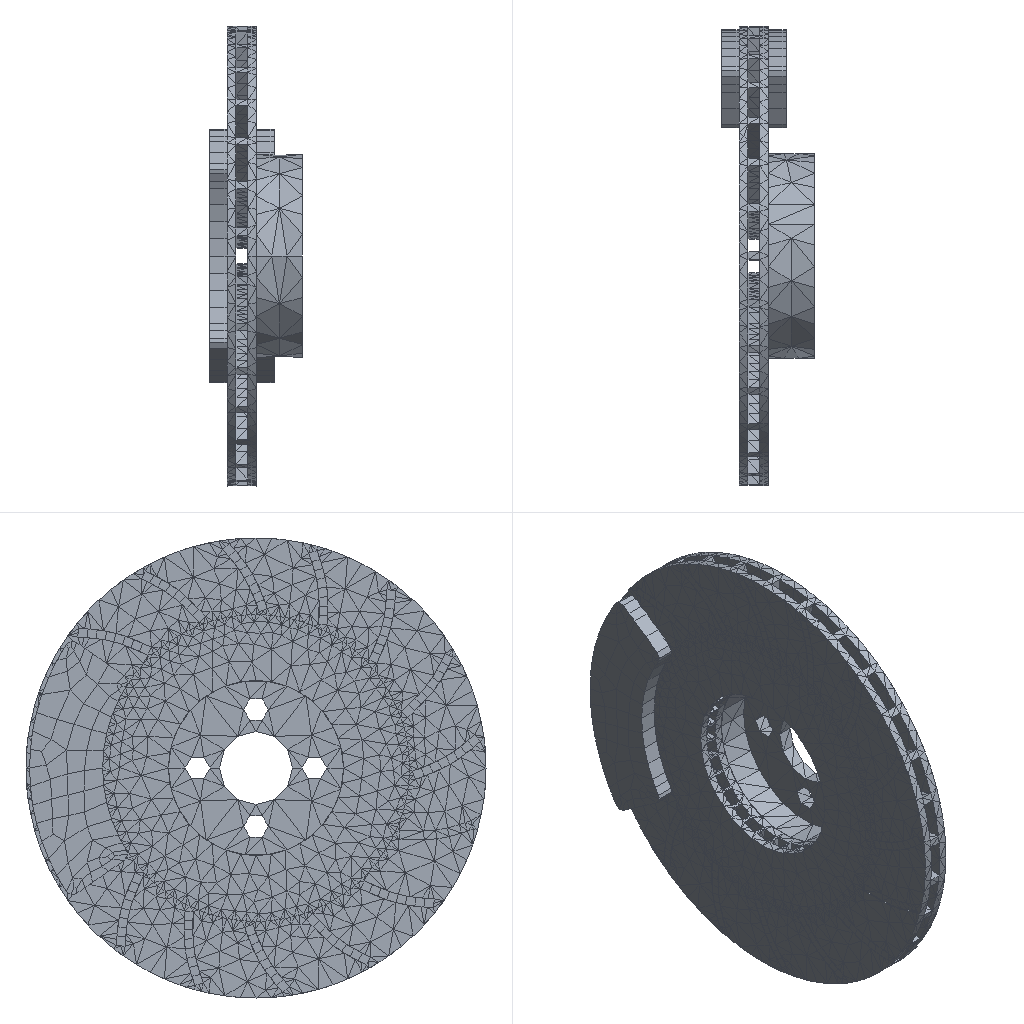Simulation study | ansys workbench
Ansys APDL input file, long lists of numbers shortened:
/batch
/config,noeldb,1     ! force off writing results to database
*get,_wallstrt,active,,time,wall
! ANSYS input file written by Workbench version 2022 R1
! File used for geometry attach:
/title,1111--___ (B5)
! ****** Begin Custom Load Command Snippet ******
/COM, ACT Extensions:
/COM,     LSDYNA, 2021.1
/COM,
! ****** End   Custom Load Command Snippet ******
*DIM,_wb_ProjectScratch_dir,string,248
_wb_ProjectScratch_dir(1) = ''
*DIM,_wb_SolverFiles_dir,string,248
_wb_SolverFiles_dir(1) = ''
*DIM,_wb_userfiles_dir,string,248
_wb_userfiles_dir(1) = ''
/com,--- Data in consistent NMM units. See Solving Units in the help system for more information.
/units,MPA
/nopr
/wb,file,start              !  signify a WB generated input file
/prep7
! Turn off shape checking because checks already performed inside WB mesher.
! See help system for more information.
SHPP,OFF,,NOWARN
/nolist
etcon,set             ! allow ANSYS to choose best KEYOP's for 180x elements, resets any applicable keyopt to MAPDL defaults
/com,*********** Nodes for the whole assembly ***********
nblock,3,,31611
(1i9,3e20.9e3)
        1    -5.687067418E+00     4.219548714E+00     4.362788327E+02
! (28737 more lines like these left out)
-1
/wb,elem,start            !  set before creation of elements
/com,*********** Elements for Body 1 "model|____-____/____1" ***********
et,1,279
eblock,19,solid,,71
(19i9)
        1        1        1        1        0        0        0        0       20        0      113     1461     1475     1498     1507     1554     1540     1517     1508
! (141 more lines like these left out)
-1
/com,*********** Elements for Body 2 "model|____-____/____1[2]" ***********
et,2,279
eblock,19,solid,,75
(19i9)
        2        2        2        2        0        0        0        0       20        0      184     2069     2116     2084     2070     2164     2117     2149     2163
! (149 more lines like these left out)
-1
/com,*********** Elements for Body 3 "model|____-____3[1]" ***********
et,3,291
eblock,19,solid,,12722
(19i9)
        3        3        3        3        0        0        0        0       10        0      763     6344     7992     7917     7984    24419    28694    24417    24418
! (25443 more lines like these left out)
-1
/com,*********** Elements for Body 4 "model|____-____3[2]" ***********
et,4,291
eblock,19,solid,,496
(19i9)
        4        4        4        4        0        0        0        0       10        0      267     2871     3008     2982     3017     3464     3916     3463     3465
! (991 more lines like these left out)
-1
/com,*********** Elements for Body 5 "model|Solid" ***********
et,5,279
eblock,19,solid,,8
(19i9)
        5        5        5        5        0        0        0        0       20        0       33      417      426      425      424      452      437      444      445
! (15 more lines like these left out)
-1
! (14 more sections like these left out)
/wb,elem,end               !  done creating elements
/com,*********** Send User Defined Coordinate System(s) ***********
csys,0
toffst,273.15,  ! Temperature offset from absolute zero
/wb,mat,start              !  starting to send materials
/com,*********** Send Materials ***********
Temperature = 'TEMP' ! Temperature
MP,DENS,1,7.85e-09,	! tonne mm^-3
MP,ALPX,1,1.2e-05,	! C^-1
MP,C,1,434000000,	! mm^2 s^-2 C^-1
MP,KXX,1,60.5,	! tonne mm s^-3 C^-1
MP,RSVX,1,0.00017,	! ohm mm
MP,EX,1,200000,	! tonne s^-2 mm^-1
MP,NUXY,1,0.3,
MP,MURX,1,10000,
Temperature = 'TEMP' ! Temperature
MP,DENS,2,7.85e-09,	! tonne mm^-3
MP,ALPX,2,1.2e-05,	! C^-1
MP,C,2,434000000,	! mm^2 s^-2 C^-1
MP,KXX,2,60.5,	! tonne mm s^-3 C^-1
MP,RSVX,2,0.00017,	! ohm mm
MP,EX,2,200000,	! tonne s^-2 mm^-1
MP,NUXY,2,0.3,
MP,MURX,2,10000,
Temperature = 'TEMP' ! Temperature
MP,DENS,3,7.85e-09,	! tonne mm^-3
MP,ALPX,3,1.2e-05,	! C^-1
MP,C,3,434000000,	! mm^2 s^-2 C^-1
MP,KXX,3,60.5,	! tonne mm s^-3 C^-1
MP,RSVX,3,0.00017,	! ohm mm
MP,EX,3,200000,	! tonne s^-2 mm^-1
MP,NUXY,3,0.3,
MP,MURX,3,10000,
Temperature = 'TEMP' ! Temperature
MP,DENS,4,7.85e-09,	! tonne mm^-3
MP,ALPX,4,1.2e-05,	! C^-1
MP,C,4,434000000,	! mm^2 s^-2 C^-1
MP,KXX,4,60.5,	! tonne mm s^-3 C^-1
MP,RSVX,4,0.00017,	! ohm mm
MP,EX,4,200000,	! tonne s^-2 mm^-1
MP,NUXY,4,0.3,
MP,MURX,4,10000,
Temperature = 'TEMP' ! Temperature
MP,DENS,5,7.85e-09,	! tonne mm^-3
MP,ALPX,5,1.2e-05,	! C^-1
MP,C,5,434000000,	! mm^2 s^-2 C^-1
MP,KXX,5,60.5,	! tonne mm s^-3 C^-1
MP,RSVX,5,0.00017,	! ohm mm
MP,EX,5,200000,	! tonne s^-2 mm^-1
MP,NUXY,5,0.3,
MP,MURX,5,10000,
Temperature = 'TEMP' ! Temperature
MP,DENS,6,7.85e-09,	! tonne mm^-3
MP,ALPX,6,1.2e-05,	! C^-1
MP,C,6,434000000,	! mm^2 s^-2 C^-1
MP,KXX,6,60.5,	! tonne mm s^-3 C^-1
MP,RSVX,6,0.00017,	! ohm mm
MP,EX,6,200000,	! tonne s^-2 mm^-1
MP,NUXY,6,0.3,
MP,MURX,6,10000,
Temperature = 'TEMP' ! Temperature
MP,DENS,7,7.85e-09,	! tonne mm^-3
MP,ALPX,7,1.2e-05,	! C^-1
MP,C,7,434000000,	! mm^2 s^-2 C^-1
MP,KXX,7,60.5,	! tonne mm s^-3 C^-1
MP,RSVX,7,0.00017,	! ohm mm
MP,EX,7,200000,	! tonne s^-2 mm^-1
MP,NUXY,7,0.3,
MP,MURX,7,10000,
Temperature = 'TEMP' ! Temperature
MP,DENS,8,7.85e-09,	! tonne mm^-3
MP,ALPX,8,1.2e-05,	! C^-1
MP,C,8,434000000,	! mm^2 s^-2 C^-1
MP,KXX,8,60.5,	! tonne mm s^-3 C^-1
MP,RSVX,8,0.00017,	! ohm mm
MP,EX,8,200000,	! tonne s^-2 mm^-1
MP,NUXY,8,0.3,
MP,MURX,8,10000,
Temperature = 'TEMP' ! Temperature
MP,DENS,9,7.85e-09,	! tonne mm^-3
MP,ALPX,9,1.2e-05,	! C^-1
MP,C,9,434000000,	! mm^2 s^-2 C^-1
MP,KXX,9,60.5,	! tonne mm s^-3 C^-1
MP,RSVX,9,0.00017,	! ohm mm
MP,EX,9,200000,	! tonne s^-2 mm^-1
! (92 more lines like these left out)
/wb,mat,end                !  done sending materials
!************************* Model Summary ********************
!model|____-____/____1,	结构钢,	matid,	1
!model|____-____/____1[2],	结构钢,	matid,	2
!model|____-____3[1],	结构钢,	matid,	3
!model|____-____3[2],	结构钢,	matid,	4
!model|Solid,	结构钢,	matid,	5
!model|Solid[2],	结构钢,	matid,	6
!model|Solid[3],	结构钢,	matid,	7
!model|Solid[4],	结构钢,	matid,	8
!model|Solid[5],	结构钢,	matid,	9
!model|Solid[6],	结构钢,	matid,	10
!model|Solid[7],	结构钢,	matid,	11
!model|Solid[8],	结构钢,	matid,	12
!model|Solid[9],	结构钢,	matid,	13
!model|Solid[10],	结构钢,	matid,	14
!model|Solid[11],	结构钢,	matid,	15
!model|Solid[12],	结构钢,	matid,	16
!model|Solid[13],	结构钢,	matid,	17
!model|Solid[14],	结构钢,	matid,	18
!model|Solid[15],	结构钢,	matid,	19
!************************* End Model Summary ********************
! get the diagonal of the bounding box. Needed later for other things
*get,_xmin,node,,mnloc,x
*get,_ymin,node,,mnloc,y
*get,_zmin,node,,mnloc,z
*get,_xmax,node,,mxloc,x
*get,_ymax,node,,mxloc,y
*get,_zmax,node,,mxloc,z
_ASMDIAG=(_xmax-_xmin)*(_xmax-_xmin)+(_ymax-_ymin)*(_ymax-_ymin)+(_zmax-_zmin)*(_zmax-_zmin)
_ASMDIAG=SQRT(_ASMDIAG)
/wb,contact,start          !  starting to send contact
/com,*********** Create Contact "接触区域" ***********
/com,            Real Constant Set For Above Contact Is 21 & 20
*set,tid,21
*set,cid,20
r,tid
r,cid
et,tid,170
et,cid,174
eblock,10,,,71
(15i9)
    22751       21       21       21        0     1554     1540     1517     1508     1908     1847     1815     1817
! (70 more lines like these left out)
-1
eblock,10,,,71
(15i9)
    22822       20       20       20        0     1554     1540     1517     1508     1908     1847     1815     1817
! (70 more lines like these left out)
-1
eblock,10,,,315
(15i9)
    22893       20       21       20        0     4246     7172     4247     4247     9933     9941     4247     9930
! (314 more lines like these left out)
-1
eblock,10,,,315
(15i9)
    23208       21       20       21        0     4246     7172     4247     4247     9933     9941     4247     9930
! (314 more lines like these left out)
-1
keyo,cid,8,2               ! auto create asymmetric contact (from Program Controlled setting)
keyo,cid,10,0              ! adjust contact stiffness each NR iteration (from Program Controlled setting)
keyo,cid,12,5              ! bonded always
keyo,cid,18,1              ! small sliding turned on by application
keyo,cid,2,0               ! augmented Lagrange (from Program Controlled setting)
keyo,cid,4,0               ! on Gauss point (from Program Controlled setting)
keyo,cid,9,1               ! ignore initial gaps/penetration
keyo,cid,7,0               ! No Prediction
rmod,tid,3,10.      ! FKN
rmod,tid,5,0.       ! ICONT
rmod,tid,6,0.       ! PINB
rmod,tid,10,0.      ! CNOF
rmod,tid,12,0.      ! FKT
rmod,tid,36,80      ! WB DSID
rmod,cid,3,10.      ! FKN
rmod,cid,5,0.       ! ICONT
rmod,cid,6,0.       ! PINB
rmod,cid,10,0.      ! CNOF
rmod,cid,12,0.      ! FKT
rmod,cid,36,80      ! WB DSID
*set,_maxkxx,605000.
rmod,cid,14,_maxkxx/_ASMDIAG         ! TCC, Divide by Length since Traction Based
rmod,tid,14,_maxkxx/_ASMDIAG      ! TCC, Divide by Length since Traction Based
keyo,cid,1,2     ! Pure thermal contact
/com,*********** Create Contact "接触区域 2" ***********
/com,            Real Constant Set For Above Contact Is 23 & 22
*set,tid,23
*set,cid,22
r,tid
r,cid
et,tid,170
et,cid,174
eblock,10,,,10
(15i9)
    23523       23       23       23        0     1512     1544     1542     1539     1831     1910     1904     1830
! (9 more lines like these left out)
-1
eblock,10,,,10
(15i9)
    23533       22       22       22        0     1512     1544     1542     1539     1831     1910     1904     1830
! (9 more lines like these left out)
-1
eblock,10,,,8
(15i9)
    23543       22       23       22        0      649      653      652      651      718      721      720      717
! (7 more lines like these left out)
-1
eblock,10,,,8
(15i9)
    23551       23       22       23        0      649      653      652      651      718      721      720      717
! (7 more lines like these left out)
-1
keyo,cid,8,2               ! auto create asymmetric contact (from Program Controlled setting)
keyo,cid,10,0              ! adjust contact stiffness each NR iteration (from Program Controlled setting)
keyo,cid,12,5              ! bonded always
keyo,cid,18,1              ! small sliding turned on by application
keyo,cid,2,0               ! augmented Lagrange (from Program Controlled setting)
keyo,cid,4,0               ! on Gauss point (from Program Controlled setting)
keyo,cid,9,1               ! ignore initial gaps/penetration
keyo,cid,7,0               ! No Prediction
rmod,tid,3,10.      ! FKN
rmod,tid,5,0.       ! ICONT
rmod,tid,6,0.       ! PINB
rmod,tid,10,0.      ! CNOF
rmod,tid,12,0.      ! FKT
rmod,tid,36,83      ! WB DSID
rmod,cid,3,10.      ! FKN
rmod,cid,5,0.       ! ICONT
rmod,cid,6,0.       ! PINB
rmod,cid,10,0.      ! CNOF
rmod,cid,12,0.      ! FKT
rmod,cid,36,83      ! WB DSID
*set,_maxkxx,605000.
rmod,cid,14,_maxkxx/_ASMDIAG         ! TCC, Divide by Length since Traction Based
rmod,tid,14,_maxkxx/_ASMDIAG      ! TCC, Divide by Length since Traction Based
keyo,cid,1,2     ! Pure thermal contact
/com,*********** Create Contact "接触区域 3" ***********
/com,            Real Constant Set For Above Contact Is 25 & 24
*set,tid,25
*set,cid,24
r,tid
r,cid
et,tid,170
et,cid,174
eblock,10,,,11
(15i9)
    23559       25       25       25        0     1529     1530     1531     1532     1881     1884     1887     1882
! (10 more lines like these left out)
-1
eblock,10,,,11
(15i9)
    23570       24       24       24        0     1529     1530     1531     1532     1881     1884     1887     1882
! (10 more lines like these left out)
-1
eblock,10,,,8
(15i9)
    23581       24       25       24        0      972      957      964      965     1021     1020     1033     1034
! (7 more lines like these left out)
-1
eblock,10,,,8
(15i9)
    23589       25       24       25        0      972      957      964      965     1021     1020     1033     1034
! (7 more lines like these left out)
-1
keyo,cid,8,2               ! auto create asymmetric contact (from Program Controlled setting)
keyo,cid,10,0              ! adjust contact stiffness each NR iteration (from Program Controlled setting)
keyo,cid,12,5              ! bonded always
keyo,cid,18,1              ! small sliding turned on by application
keyo,cid,2,0               ! augmented Lagrange (from Program Controlled setting)
keyo,cid,4,0               ! on Gauss point (from Program Controlled setting)
keyo,cid,9,1               ! ignore initial gaps/penetration
keyo,cid,7,0               ! No Prediction
rmod,tid,3,10.      ! FKN
rmod,tid,5,0.       ! ICONT
rmod,tid,6,0.       ! PINB
rmod,tid,10,0.      ! CNOF
rmod,tid,12,0.      ! FKT
rmod,tid,36,86      ! WB DSID
rmod,cid,3,10.      ! FKN
rmod,cid,5,0.       ! ICONT
rmod,cid,6,0.       ! PINB
rmod,cid,10,0.      ! CNOF
rmod,cid,12,0.      ! FKT
rmod,cid,36,86      ! WB DSID
*set,_maxkxx,605000.
rmod,cid,14,_maxkxx/_ASMDIAG         ! TCC, Divide by Length since Traction Based
rmod,tid,14,_maxkxx/_ASMDIAG      ! TCC, Divide by Length since Traction Based
keyo,cid,1,2     ! Pure thermal contact
/com,*********** Create Contact "接触区域 4" ***********
/com,            Real Constant Set For Above Contact Is 27 & 26
*set,tid,27
*set,cid,26
r,tid
r,cid
et,tid,170
et,cid,174
eblock,10,,,14
(15i9)
    23597       27       27       27        0     1554     1540     1517     1508     1908     1847     1815     1817
! (13 more lines like these left out)
-1
eblock,10,,,14
(15i9)
    23611       26       26       26        0     1554     1540     1517     1508     1908     1847     1815     1817
! (13 more lines like these left out)
-1
eblock,10,,,8
(15i9)
    23625       26       27       26        0      337      341      340      339      406      409      408      405
! (7 more lines like these left out)
-1
eblock,10,,,8
(15i9)
    23633       27       26       27        0      337      341      340      339      406      409      408      405
! (7 more lines like these left out)
-1
keyo,cid,8,2               ! auto create asymmetric contact (from Program Controlled setting)
keyo,cid,10,0              ! adjust contact stiffness each NR iteration (from Program Controlled setting)
keyo,cid,12,5              ! bonded always
keyo,cid,18,1              ! small sliding turned on by application
keyo,cid,2,0               ! augmented Lagrange (from Program Controlled setting)
keyo,cid,4,0               ! on Gauss point (from Program Controlled setting)
keyo,cid,9,1               ! ignore initial gaps/penetration
keyo,cid,7,0               ! No Prediction
rmod,tid,3,10.      ! FKN
rmod,tid,5,0.       ! ICONT
rmod,tid,6,0.       ! PINB
rmod,tid,10,0.      ! CNOF
rmod,tid,12,0.      ! FKT
rmod,tid,36,89      ! WB DSID
rmod,cid,3,10.      ! FKN
rmod,cid,5,0.       ! ICONT
rmod,cid,6,0.       ! PINB
rmod,cid,10,0.      ! CNOF
rmod,cid,12,0.      ! FKT
rmod,cid,36,89      ! WB DSID
*set,_maxkxx,605000.
rmod,cid,14,_maxkxx/_ASMDIAG         ! TCC, Divide by Length since Traction Based
rmod,tid,14,_maxkxx/_ASMDIAG      ! TCC, Divide by Length since Traction Based
keyo,cid,1,2     ! Pure thermal contact
/com,*********** Create Contact "接触区域 5" ***********
/com,            Real Constant Set For Above Contact Is 29 & 28
*set,tid,29
*set,cid,28
r,tid
r,cid
et,tid,170
et,cid,174
eblock,10,,,75
(15i9)
    23641       29       29       29        0     2149     2163     2164     2117     2531     2556     2443     2442
! (74 more lines like these left out)
-1
eblock,10,,,75
(15i9)
    23716       28       28       28        0     2149     2163     2164     2117     2531     2556     2443     2442
! (74 more lines like these left out)
-1
eblock,10,,,315
(15i9)
    23791       28       29       28        0     7277     7307     7294     7294    27401    27483     7294    27400
! (314 more lines like these left out)
-1
eblock,10,,,315
(15i9)
    24106       29       28       29        0     7277     7307     7294     7294    27401    27483     7294    27400
! (314 more lines like these left out)
-1
keyo,cid,8,2               ! auto create asymmetric contact (from Program Controlled setting)
keyo,cid,10,0              ! adjust contact stiffness each NR iteration (from Program Controlled setting)
keyo,cid,12,5              ! bonded always
keyo,cid,18,1              ! small sliding turned on by application
keyo,cid,2,0               ! augmented Lagrange (from Program Controlled setting)
keyo,cid,4,0               ! on Gauss point (from Program Controlled setting)
keyo,cid,9,1               ! ignore initial gaps/penetration
keyo,cid,7,0               ! No Prediction
rmod,tid,3,10.      ! FKN
rmod,tid,5,0.       ! ICONT
rmod,tid,6,0.       ! PINB
rmod,tid,10,0.      ! CNOF
rmod,tid,12,0.      ! FKT
rmod,tid,36,92      ! WB DSID
rmod,cid,3,10.      ! FKN
rmod,cid,5,0.       ! ICONT
rmod,cid,6,0.       ! PINB
rmod,cid,10,0.      ! CNOF
rmod,cid,12,0.      ! FKT
rmod,cid,36,92      ! WB DSID
*set,_maxkxx,605000.
rmod,cid,14,_maxkxx/_ASMDIAG         ! TCC, Divide by Length since Traction Based
rmod,tid,14,_maxkxx/_ASMDIAG      ! TCC, Divide by Length since Traction Based
keyo,cid,1,2     ! Pure thermal contact
! (16 more sections like these left out)
/wb,contact,end            !  done creating contacts
/golist
/wb,load,start             !  starting to send loads
/com,*********** Define Temperature Constraint ***********
CMBLOCK,_CM151  ,NODE,     4828
(8i10)
      3963      3965      3966      3967      3968      3969      3970      3971
! (603 more lines like these left out)
fcum,add                   ! add nodal forces up (needed in case have loads on the same edge,vertex)
fcum                       ! reset default on fcum command since done sending WB F loads
/com,*********** Create "______" ***********
et,62,152
eblock,10,,,1858
(15i9)
    27047       62       62       62        0     7290     7335     7298     7298    27465    27498     7298    27463
! (1857 more lines like these left out)
-1
esel,s,type,,62
keyop,62,8,2.
keyop,62,13,0
esel,all
/com,***************** Define Uniform Initial temperature ***************
tunif,22.
/gst,on,on
fini
*get,_numnode,node,0,count
*get,_numelem,elem,0,count
*get, _MAXELEMNUM, elem, 0, NUM, MAX
*get, _MAXNODENUM, node, 0, NUM, MAX
*get, _MAXELEMTYPE, etyp, 0, NUM, MAX
*get, _MAXREALCONST, real, 0, NUM, MAX
/go
/wb,load,end               !  done creating loads
/com,--- Number of total nodes = %_numnode%
/com,--- Number of contact elements = 6154
/com,--- Number of spring elements = 0
/com,--- Number of bearing elements = 0
/com,--- Number of solid elements = 13484
/com,--- Number of condensed parts = 0
/com,--- Number of total elements = %_numelem%
*get,_wallbsol,active,,time,wall
/com,****************************************************************************
/com,*************************    SOLUTION       ********************************
/com,****************************************************************************
/solu
antype,4                   ! transient analysis
kbc,1                      ! stepped BC's
!eqsl,sparse               ! using sparse solver which is default so no eqsl command needed
cntr,print,1               ! print out contact info and also make no initial contact an error
rescontrol,,none                 ! Do not keep any restart files
dmpoption,emat,no             ! Don't combine emat file for DANSYS
dmpoption,esav,no             ! Don't combine esav file for DANSYS
thopt,quasi,5.e-002
nlhist,nsol,MAX_TEMP,temp,max
nlhist,nsol,MIN_TEMP,temp,min
/com,********* Initial Time Increment Check And Fourier Modulus *********
/com, Specified Initial Time Increment: 0.01
/com, Estimated Increment Needed, le*le/alpha, Body 1: 6.84
/com, Estimated Increment Needed, le*le/alpha, Body 2: 6.594
/com, Estimated Increment Needed, le*le/alpha, Body 3: 0.9474
/com, Estimated Increment Needed, le*le/alpha, Body 4: 3.206
/com, Estimated Increment Needed, le*le/alpha, Body 5: 0.6388
/com, Estimated Increment Needed, le*le/alpha, Body 6: 0.6388
/com, Estimated Increment Needed, le*le/alpha, Body 7: 0.6388
/com, Estimated Increment Needed, le*le/alpha, Body 8: 0.6388
/com, Estimated Increment Needed, le*le/alpha, Body 9: 0.6388
/com, Estimated Increment Needed, le*le/alpha, Body 10: 0.6388
/com, Estimated Increment Needed, le*le/alpha, Body 11: 0.6388
/com, Estimated Increment Needed, le*le/alpha, Body 12: 0.6388
/com, Estimated Increment Needed, le*le/alpha, Body 13: 0.6388
/com, Estimated Increment Needed, le*le/alpha, Body 14: 0.6388
/com, Estimated Increment Needed, le*le/alpha, Body 15: 0.6388
/com, Estimated Increment Needed, le*le/alpha, Body 16: 0.6388
/com, Estimated Increment Needed, le*le/alpha, Body 17: 0.6388
/com, Estimated Increment Needed, le*le/alpha, Body 18: 0.6388
/com, Estimated Increment Needed, le*le/alpha, Body 19: 0.6388
/com,****************************************************
/com,******************* SOLVE FOR LS 1 OF 1 ****************
d,_CM151,temp,200.
esel,s,type,,62
nsle
sf,all,conv,15000.,22.
nsel,all
esel,all
/nopr
/gopr
autots,on
nsub,100,1000,10
time,1.
timint,on                  ! Turn on time integration effects
outres,erase
outres,all,none
outres,nsol,all
outres,rsol,all
outres,eangl,all
outres,veng,all
outres,fflux,all
outres,cont,all
/nopr
esel,s,type,,62
cm,_elmisc,elem
esel,all
/gopr
outres,misc,all,_elmisc
cnvtol,heat,,.001,,1.e-003    ! Program Controlled. Set MINREF equivalent of 1e-6 Watts
! *********** WB SOLVE COMMAND ***********
! check interactive state
*get,ANSINTER_,active,,int
*if,ANSINTER_,ne,0,then
/eof
*endif
solve
/com *************** Write FE CONNECTORS *********
CEWRITE,file,ce,,INTE
/com,****************************************************
/com,*************** FINISHED SOLVE FOR LS 1 *************
*get,_wallasol,active,,time,wall
/post1
xmlo,ENCODING,ISO-8859-1
xmlo,parm
/xml,parm,xml
fini
/gopr
*get,_walldone,active,,time,wall
_preptime=(_wallbsol-_wallstrt)*3600
_solvtime=(_wallasol-_wallbsol)*3600
_posttime=(_walldone-_wallasol)*3600
_totaltim=(_walldone-_wallstrt)*3600
*get,_dlbratio,active,0,solu,dlbr
*get,_combtime,active,0,solu,comb
*get,_ssmode,active,0,solu,ssmm
*get,_ndofs,active,0,solu,ndof
/fclean				!clean distributed files
/com,--- Total number of nodes = %_numnode%
/com,--- Total number of elements = %_numelem%
/com,--- Element load balance ratio = %_dlbratio%
/com,--- Time to combine distributed files = %_combtime%
/com,--- Sparse memory mode = %_ssmode%
/com,--- Number of DOF = %_ndofs%
/wb,file,end               ! done with WB generated input